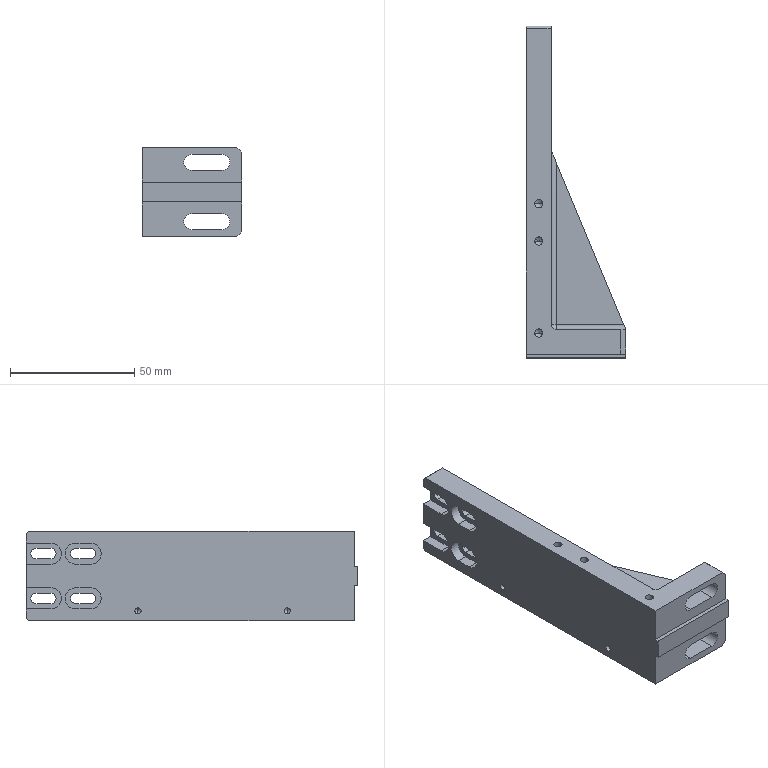Part | SolidWorks | features ICE 5, HoleWzd 3, Chamfer 2, Cut 1, Extrusion 1, Fillet 1, MirrorPattern 1, Rib 1 | 1 solid | 108 faces | box 40 x 133.5 x 36 mm | volume 59934 mm3 | plane 48 | cylinder 46 | cone 12 | sphere 2 | commonest cylinder face diameters 4.2 x12 8.5 x10 3.3 x8 4 x6 2.5 x4 6.5 x4